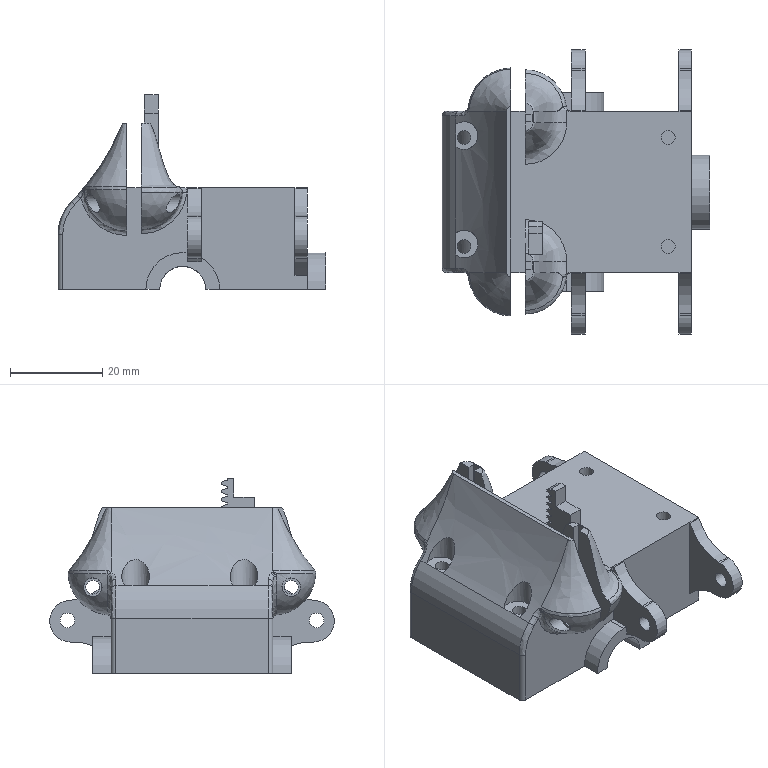Part | STEP file | Wytnij-wyci_gni_cie6 | 1 solid | 267 faces | box 58 x 61.646 x 42.232 mm | volume 26812 mm3 | plane 122 | cylinder 109 | spline 36 | commonest cylinder face diameters 0.119 x22 0.199 x22 3 x12 16 x10 20 x8 8 x6